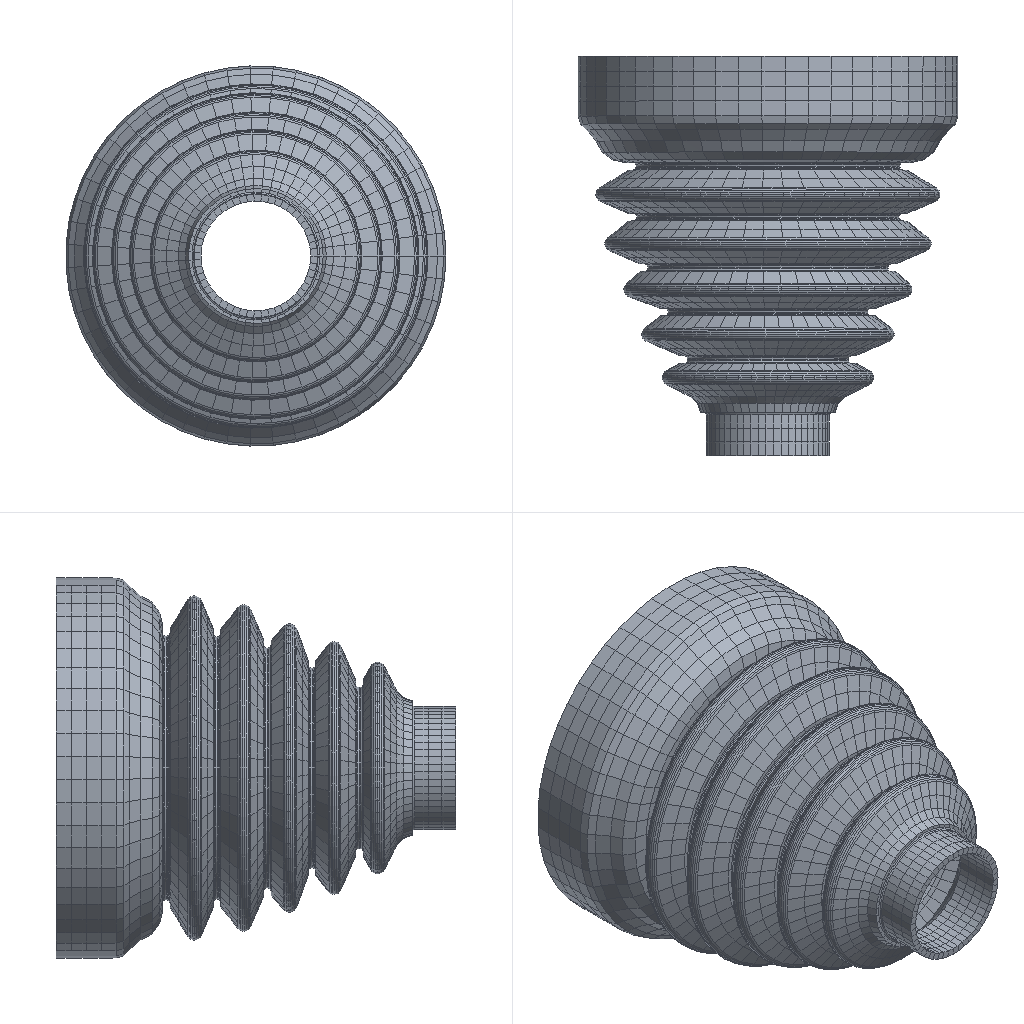Simulation study | abaqus
Set-up summary:
category,name,step,type,value,unit,region
solver,abaqus,,Abaqus/CAE 2024
units,unstated,,unstated
analysis,Step-1,,static,nlgeom=True; time_period=1
analysis,Step-2,,static,nlgeom=True; time_period=1
mesh,nodes,,,62019
mesh,elements,,,11731
element_type,C3D20H,,,11730
element_type,CONN3D2,,,1
material,MATERIAL-1,,behaviors,hyperelastic; viscoelastic
section,MATERIAL-1,,solid section,,,SET-2
bc,BC-5,Step-1,fixed,"[dofs=rx,ry,rz,x,y,z n=6]",,_PickedSet80
bc,BC-5-Copy,Step-1,fixed,"[dofs=rx,ry,rz,x,y,z n=6]",,_PickedSet79
bc,BC-5,Step-2,displacement,0.75 [dofs=ry],,_PickedSet80
bc,BC-5-Copy,Step-2,displacement,0.75 [dofs=ry],,_PickedSet79
bc,BC-7,Step-2,fixed,"[dofs=rx,rz,x,y,z n=5]",,_PickedSet78
bc,BC-7,Step-2,displacement,0.75 [dofs=ry],,_PickedSet78
contact,Int-2,initial,general contact,interaction=INTPROP-1; friction=0.3; behavior=hard
constraint,connector section,,,1
constraint,coupling,,,2
Abaqus input file, long lists of numbers shortened:
*Heading
** Job name: deck Model name: Job-1-Copy-Copy
** Generated by: Abaqus/CAE 2024
*Preprint, echo=NO, model=NO, history=NO, contact=NO
**
** PARTS
**
*Part, name=PART-1-1
*Node
      1,         14.5,        -122.,           0.
      2,         14.5,  -109.9,           0.
** (62014 more lines like these left out)
*Element, type=C3D20H
    1,    156,      1,    157,    196,    485,    330,    486,    525,  62020,  62019,  62018,  62017,  62021,  62022,  62023,
        62024,  62026,  62025,  62027,  62028
** (23458 more lines like these left out)
*Nset, nset=SET-1, generate
     1,  16779,      1
*Elset, elset=SET-1, generate
     1,  11730,      1
*Nset, nset=SET-2, generate
     1,  16779,      1
*Elset, elset=SET-2, generate
     1,  11730,      1
** Section: Section-1-SET-2
*Solid Section, elset=SET-2, material=MATERIAL-1
,
*End Part
**
**
** ASSEMBLY
**
*Assembly, name=Assembly
**
*Instance, name=PART-1-1, part=PART-1-1
*End Instance
**
*Node
      3,           0.,           0.,           0.
*Node
      1,           0.,        -116.,           0.
      2,           0.,         -25.,           0.
*Element, type=CONN3D2
1, 1, 3
*Connector Section, elset=Wire-1-Set-2
Hinge,
"Datum csys-1",
*Nset, nset=M_SET-1
 1,
*Nset, nset=M_SET-8
 1,
*Nset, nset=M_SET-10
 2,
*Nset, nset=M_SET-14
 1,
*Nset, nset=M_SET-16
 2,
*Nset, nset=M_SET-21, instance=PART-1-1
    53,    54,   170,   171,   172,   382,   383,   499,   500,   501,   711,   712,   828,   829,   830,  1040
  1041,  1157,  1158,  1159,  1369,  1370,  1486,  1487,  1488,  1698,  1699,  1815,  1816,  1817,  2027,  2028
** (14 more lines like these left out)
*Elset, elset=M_SET-21, instance=PART-1-1
    91,    92,   120,   121,   321,   322,   350,   351,   551,   552,   580,   581,   781,   782,   810,   811
  1011,  1012,  1040,  1041,  1241,  1242,  1270,  1271,  1471,  1472,  1500,  1501,  1701,  1702,  1730,  1731
** (11 more lines like these left out)
*Nset, nset=M_SET-27
 1,
*Nset, nset=M_SET-29
 2,
*Nset, nset=SET-3, instance=PART-1-1
    55,    56,   173,   174,   175,   384,   385,   502,   503,   504,   713,   714,   831,   832,   833,  1042
  1043,  1160,  1161,  1162,  1371,  1372,  1489,  1490,  1491,  1700,  1701,  1818,  1819,  1820,  2029,  2030
** (14 more lines like these left out)
*Elset, elset=SET-3, instance=PART-1-1
    91,    92,   120,   121,   321,   322,   350,   351,   551,   552,   580,   581,   781,   782,   810,   811
  1011,  1012,  1040,  1041,  1241,  1242,  1270,  1271,  1471,  1472,  1500,  1501,  1701,  1702,  1730,  1731
** (11 more lines like these left out)
*Nset, nset=SET-4
 1,
*Nset, nset=SET-5, instance=PART-1-1, generate
     1,  16779,      1
*Nset, nset=SET-5
 1,
*Elset, elset=SET-5, instance=PART-1-1, generate
     1,  11730,      1
*Nset, nset=SET-7, instance=PART-1-1
     1,     2,   157,   158,   159,   330,   331,   486,   487,   488,   659,   660,   815,   816,   817,   988
   989,  1144,  1145,  1146,  1317,  1318,  1473,  1474,  1475,  1646,  1647,  1802,  1803,  1804,  1975,  1976
** (14 more lines like these left out)
*Elset, elset=SET-7, instance=PART-1-1
     1,     2,   110,   177,   231,   232,   340,   407,   461,   462,   570,   637,   691,   692,   800,   867
   921,   922,  1030,  1097,  1151,  1152,  1260,  1327,  1381,  1382,  1490,  1557,  1611,  1612,  1720,  1787
** (11 more lines like these left out)
*Nset, nset=SET-12
 1,
*Nset, nset=SET-13, instance=PART-1-1
    53,    54,   170,   171,   172,   382,   383,   499,   500,   501,   711,   712,   828,   829,   830,  1040
  1041,  1157,  1158,  1159,  1369,  1370,  1486,  1487,  1488,  1698,  1699,  1815,  1816,  1817,  2027,  2028
** (14 more lines like these left out)
*Elset, elset=SET-13, instance=PART-1-1
    91,    92,   120,   121,   321,   322,   350,   351,   551,   552,   580,   581,   781,   782,   810,   811
  1011,  1012,  1040,  1041,  1241,  1242,  1270,  1271,  1471,  1472,  1500,  1501,  1701,  1702,  1730,  1731
** (11 more lines like these left out)
*Nset, nset=SET-18
 1,
*Nset, nset=SET-19, instance=PART-1-1
     1,     2,   157,   158,   159,   330,   331,   486,   487,   488,   659,   660,   815,   816,   817,   988
   989,  1144,  1145,  1146,  1317,  1318,  1473,  1474,  1475,  1646,  1647,  1802,  1803,  1804,  1975,  1976
** (14 more lines like these left out)
*Elset, elset=SET-19, instance=PART-1-1
     1,     2,   110,   177,   231,   232,   340,   407,   461,   462,   570,   637,   691,   692,   800,   867
   921,   922,  1030,  1097,  1151,  1152,  1260,  1327,  1381,  1382,  1490,  1557,  1611,  1612,  1720,  1787
** (11 more lines like these left out)
*Nset, nset=SET-20, instance=PART-1-1
    53,    54,   170,   171,   172,   382,   383,   499,   500,   501,   711,   712,   828,   829,   830,  1040
  1041,  1157,  1158,  1159,  1369,  1370,  1486,  1487,  1488,  1698,  1699,  1815,  1816,  1817,  2027,  2028
** (14 more lines like these left out)
*Elset, elset=SET-20, instance=PART-1-1
    91,    92,   120,   121,   321,   322,   350,   351,   551,   552,   580,   581,   781,   782,   810,   811
  1011,  1012,  1040,  1041,  1241,  1242,  1270,  1271,  1471,  1472,  1500,  1501,  1701,  1702,  1730,  1731
** (11 more lines like these left out)
*Nset, nset=SET-23, instance=PART-1-1
    53,    54,   170,   171,   172,   382,   383,   499,   500,   501,   711,   712,   828,   829,   830,  1040
  1041,  1157,  1158,  1159,  1369,  1370,  1486,  1487,  1488,  1698,  1699,  1815,  1816,  1817,  2027,  2028
** (14 more lines like these left out)
*Elset, elset=SET-23, instance=PART-1-1
    91,    92,   120,   121,   321,   322,   350,   351,   551,   552,   580,   581,   781,   782,   810,   811
  1011,  1012,  1040,  1041,  1241,  1242,  1270,  1271,  1471,  1472,  1500,  1501,  1701,  1702,  1730,  1731
** (11 more lines like these left out)
*Nset, nset=SET-24, instance=PART-1-1
     1,     2,   157,   158,   159,   330,   331,   486,   487,   488,   659,   660,   815,   816,   817,   988
   989,  1144,  1145,  1146,  1317,  1318,  1473,  1474,  1475,  1646,  1647,  1802,  1803,  1804,  1975,  1976
** (14 more lines like these left out)
*Elset, elset=SET-24, instance=PART-1-1
     1,     2,   110,   177,   231,   232,   340,   407,   461,   462,   570,   637,   691,   692,   800,   867
   921,   922,  1030,  1097,  1151,  1152,  1260,  1327,  1381,  1382,  1490,  1557,  1611,  1612,  1720,  1787
** (11 more lines like these left out)
*Nset, nset=SET-31, instance=PART-1-1, generate
     1,  16779,      1
*Nset, nset=SET-31
 1, 2
*Elset, elset=SET-31, instance=PART-1-1, generate
     1,  11730,      1
*Nset, nset=SET-44
 1,
*Nset, nset=S_SET-1, instance=PART-1-1
     1,     2,   157,   158,   159,   330,   331,   486,   487,   488,   659,   660,   815,   816,   817,   988
   989,  1144,  1145,  1146,  1317,  1318,  1473,  1474,  1475,  1646,  1647,  1802,  1803,  1804,  1975,  1976
** (14 more lines like these left out)
*Elset, elset=S_SET-1, instance=PART-1-1
     1,     2,   110,   177,   231,   232,   340,   407,   461,   462,   570,   637,   691,   692,   800,   867
   921,   922,  1030,  1097,  1151,  1152,  1260,  1327,  1381,  1382,  1490,  1557,  1611,  1612,  1720,  1787
** (11 more lines like these left out)
*Nset, nset=S_SET-8, instance=PART-1-1
     1,     2,   157,   158,   159,   330,   331,   486,   487,   488,   659,   660,   815,   816,   817,   988
   989,  1144,  1145,  1146,  1317,  1318,  1473,  1474,  1475,  1646,  1647,  1802,  1803,  1804,  1975,  1976
** (14 more lines like these left out)
*Elset, elset=S_SET-8, instance=PART-1-1
     1,     2,   110,   177,   231,   232,   340,   407,   461,   462,   570,   637,   691,   692,   800,   867
   921,   922,  1030,  1097,  1151,  1152,  1260,  1327,  1381,  1382,  1490,  1557,  1611,  1612,  1720,  1787
** (11 more lines like these left out)
*Nset, nset=S_SET-10, instance=PART-1-1
    53,    54,   170,   171,   172,   382,   383,   499,   500,   501,   711,   712,   828,   829,   830,  1040
  1041,  1157,  1158,  1159,  1369,  1370,  1486,  1487,  1488,  1698,  1699,  1815,  1816,  1817,  2027,  2028
** (14 more lines like these left out)
*Elset, elset=S_SET-10, instance=PART-1-1
    91,    92,   120,   121,   321,   322,   350,   351,   551,   552,   580,   581,   781,   782,   810,   811
  1011,  1012,  1040,  1041,  1241,  1242,  1270,  1271,  1471,  1472,  1500,  1501,  1701,  1702,  1730,  1731
** (11 more lines like these left out)
*Nset, nset=S_SET-14, instance=PART-1-1
     1,     2,   157,   158,   159,   330,   331,   486,   487,   488,   659,   660,   815,   816,   817,   988
   989,  1144,  1145,  1146,  1317,  1318,  1473,  1474,  1475,  1646,  1647,  1802,  1803,  1804,  1975,  1976
** (14 more lines like these left out)
*Elset, elset=S_SET-14, instance=PART-1-1
     1,     2,   110,   177,   231,   232,   340,   407,   461,   462,   570,   637,   691,   692,   800,   867
   921,   922,  1030,  1097,  1151,  1152,  1260,  1327,  1381,  1382,  1490,  1557,  1611,  1612,  1720,  1787
** (11 more lines like these left out)
*Nset, nset=S_SET-16, instance=PART-1-1
    53,    54,   170,   171,   172,   382,   383,   499,   500,   501,   711,   712,   828,   829,   830,  1040
  1041,  1157,  1158,  1159,  1369,  1370,  1486,  1487,  1488,  1698,  1699,  1815,  1816,  1817,  2027,  2028
** (14 more lines like these left out)
*Elset, elset=S_SET-16, instance=PART-1-1
    91,    92,   120,   121,   321,   322,   350,   351,   551,   552,   580,   581,   781,   782,   810,   811
  1011,  1012,  1040,  1041,  1241,  1242,  1270,  1271,  1471,  1472,  1500,  1501,  1701,  1702,  1730,  1731
** (11 more lines like these left out)
*Nset, nset=S_SET-21
 2,
*Nset, nset=S_SET-27, instance=PART-1-1
     1,     2,   157,   158,   159,   330,   331,   486,   487,   488,   659,   660,   815,   816,   817,   988
   989,  1144,  1145,  1146,  1317,  1318,  1473,  1474,  1475,  1646,  1647,  1802,  1803,  1804,  1975,  1976
** (14 more lines like these left out)
*Elset, elset=S_SET-27, instance=PART-1-1
     1,     2,   110,   177,   231,   232,   340,   407,   461,   462,   570,   637,   691,   692,   800,   867
   921,   922,  1030,  1097,  1151,  1152,  1260,  1327,  1381,  1382,  1490,  1557,  1611,  1612,  1720,  1787
** (11 more lines like these left out)
*Nset, nset=S_SET-29, instance=PART-1-1
    53,    54,   170,   171,   172,   382,   383,   499,   500,   501,   711,   712,   828,   829,   830,  1040
  1041,  1157,  1158,  1159,  1369,  1370,  1486,  1487,  1488,  1698,  1699,  1815,  1816,  1817,  2027,  2028
** (14 more lines like these left out)
*Elset, elset=S_SET-29, instance=PART-1-1
    91,    92,   120,   121,   321,   322,   350,   351,   551,   552,   580,   581,   781,   782,   810,   811
  1011,  1012,  1040,  1041,  1241,  1242,  1270,  1271,  1471,  1472,  1500,  1501,  1701,  1702,  1730,  1731
** (11 more lines like these left out)
*Nset, nset=Wire-1-Set-2
 1, 3
*Elset, elset=Wire-1-Set-2
 1,
*Nset, nset=S_SET-27_CNS_, internal, instance=PART-1-1
     1,     2,   157,   158,   159,   330,   331,   486,   487,   488,   659,   660,   815,   816,   817,   988
   989,  1144,  1145,  1146,  1317,  1318,  1473,  1474,  1475,  1646,  1647,  1802,  1803,  1804,  1975,  1976
** (14 more lines like these left out)
*Nset, nset=S_SET-29_CNS_, internal, instance=PART-1-1
    53,    54,   170,   171,   172,   382,   383,   499,   500,   501,   711,   712,   828,   829,   830,  1040
  1041,  1157,  1158,  1159,  1369,  1370,  1486,  1487,  1488,  1698,  1699,  1815,  1816,  1817,  2027,  2028
** (14 more lines like these left out)
*Nset, nset=_PickedSet68, internal
 2,
*Nset, nset=_PickedSet73, internal
 3,
*Nset, nset=_PickedSet77, internal
 1,
*Nset, nset=_PickedSet78, internal
 1,
*Nset, nset=_PickedSet79, internal
 2,
*Nset, nset=_PickedSet80, internal
 3,
*Elset, elset=_PickedSet81, internal
 1,
*Elset, elset=_SURF-1_S3, internal, instance=PART-1-1
     1,     5,     8,    14,    19,    20,    26,    33,    53,    56,    57,    59,    64,    89,    93,    95
    98,   100,   101,   106,   113,   115,   118,   133,   144,   152,   160,   161,   162,   163,   165,   167
** (139 more lines like these left out)
*Elset, elset=_SURF-1_S4, internal, instance=PART-1-1
     1,     2,     6,     7,    10,    17,    18,    21,    27,    31,    43,    45,    47,    52,    55,    58
    62,    66,    69,    77,    81,    87,    88,    90,    91,    92,    96,   104,   107,   109,   110,   114
** (180 more lines like these left out)
*Elset, elset=_SURF-1_S5, internal, instance=PART-1-1
     4,     9,    11,    15,    16,    24,    29,    32,    34,    36,    37,    42,    46,    49,    53,    60
    61,    67,    73,    82,    85,    89,    93,    95,   102,   103,   111,   113,   121,   130,   132,   137
** (142 more lines like these left out)
*Elset, elset=_SURF-1_S6, internal, instance=PART-1-1
     1,     2,     3,     5,     6,     7,    13,    22,    30,    39,    44,    50,    51,    52,    54,    63
    65,    68,    70,    71,    74,    78,    79,    83,    84,    86,    88,    90,    91,    92,    99,   109
** (158 more lines like these left out)
*Elset, elset=_SURF-2_S3, internal, instance=PART-1-1
     1,     5,     8,    14,    19,    20,    26,    33,    53,    56,    57,    59,    64,    89,    93,    95
    98,   100,   101,   106,   113,   115,   118,   133,   144,   152,   160,   161,   162,   163,   165,   167
** (139 more lines like these left out)
*Elset, elset=_SURF-2_S4, internal, instance=PART-1-1
     1,     2,     6,     7,    10,    17,    18,    21,    27,    31,    43,    45,    47,    52,    55,    58
    62,    66,    69,    77,    81,    87,    88,    90,    91,    92,    96,   104,   107,   109,   110,   114
** (180 more lines like these left out)
*Elset, elset=_SURF-2_S5, internal, instance=PART-1-1
     4,     9,    11,    15,    16,    24,    29,    32,    34,    36,    37,    42,    46,    49,    53,    60
    61,    67,    73,    82,    85,    89,    93,    95,   102,   103,   111,   113,   121,   130,   132,   137
** (142 more lines like these left out)
*Elset, elset=_SURF-2_S6, internal, instance=PART-1-1
     1,     2,     3,     5,     6,     7,    13,    22,    30,    39,    44,    50,    51,    52,    54,    63
    65,    68,    70,    71,    74,    78,    79,    83,    84,    86,    88,    90,    91,    92,    99,   109
** (158 more lines like these left out)
*Elset, elset=_SURF-1_S3_1, internal, instance=PART-1-1
     1,     5,     8,    14,    19,    20,    26,    33,    53,    56,    57,    59,    64,    89,    93,    95
    98,   100,   101,   106,   113,   115,   118,   133,   144,   152,   160,   161,   162,   163,   165,   167
** (139 more lines like these left out)
*Elset, elset=_SURF-1_S4_1, internal, instance=PART-1-1
     1,     2,     6,     7,    10,    17,    18,    21,    27,    31,    43,    45,    47,    52,    55,    58
    62,    66,    69,    77,    81,    87,    88,    90,    91,    92,    96,   104,   107,   109,   110,   114
** (180 more lines like these left out)
*Elset, elset=_SURF-1_S6_1, internal, instance=PART-1-1
     1,     2,     3,     5,     6,     7,    13,    22,    30,    39,    44,    50,    51,    52,    54,    63
    65,    68,    70,    71,    74,    78,    79,    83,    84,    86,    88,    90,    91,    92,    99,   109
** (158 more lines like these left out)
*Elset, elset=_SURF-1_S5_1, internal, instance=PART-1-1
     4,     9,    11,    15,    16,    24,    29,    32,    34,    36,    37,    42,    46,    49,    53,    60
    61,    67,    73,    82,    85,    89,    93,    95,   102,   103,   111,   113,   121,   130,   132,   137
** (142 more lines like these left out)
*Surface, type=ELEMENT, name=SURF-1
_SURF-1_S3_1, S3
_SURF-1_S4_1, S4
_SURF-1_S6_1, S6
_SURF-1_S5_1, S5
*Elset, elset=_SURF-2_S3_1, internal, instance=PART-1-1
     1,     5,     8,    14,    19,    20,    26,    33,    53,    56,    57,    59,    64,    89,    93,    95
    98,   100,   101,   106,   113,   115,   118,   133,   144,   152,   160,   161,   162,   163,   165,   167
** (139 more lines like these left out)
*Elset, elset=_SURF-2_S4_1, internal, instance=PART-1-1
     1,     2,     6,     7,    10,    17,    18,    21,    27,    31,    43,    45,    47,    52,    55,    58
    62,    66,    69,    77,    81,    87,    88,    90,    91,    92,    96,   104,   107,   109,   110,   114
** (180 more lines like these left out)
*Elset, elset=_SURF-2_S6_1, internal, instance=PART-1-1
     1,     2,     3,     5,     6,     7,    13,    22,    30,    39,    44,    50,    51,    52,    54,    63
    65,    68,    70,    71,    74,    78,    79,    83,    84,    86,    88,    90,    91,    92,    99,   109
** (158 more lines like these left out)
*Elset, elset=_SURF-2_S5_1, internal, instance=PART-1-1
     4,     9,    11,    15,    16,    24,    29,    32,    34,    36,    37,    42,    46,    49,    53,    60
    61,    67,    73,    82,    85,    89,    93,    95,   102,   103,   111,   113,   121,   130,   132,   137
** (142 more lines like these left out)
*Surface, type=ELEMENT, name=SURF-2
_SURF-2_S3_1, S3
_SURF-2_S4_1, S4
_SURF-2_S6_1, S6
_SURF-2_S5_1, S5
*Surface, type=NODE, name=S_SET-27_CNS__CNS_, internal
S_SET-27_CNS_, 1.
*Surface, type=NODE, name=S_SET-29_CNS__CNS_, internal
S_SET-29_CNS_, 1.
*Orientation, name="Datum csys-1"
          1.,           0.,           0.,           0.,           1.,           0.
1, 0.
** Constraint: CONSTRAINT-1
*Coupling, constraint name=CONSTRAINT-1, ref node=M_SET-27, surface=S_SET-27_CNS__CNS_
*Kinematic
** Constraint: CONSTRAINT-2
*Coupling, constraint name=CONSTRAINT-2, ref node=M_SET-29, surface=S_SET-29_CNS__CNS_
*Kinematic
1, 1
2, 2
3, 3
4, 4
6, 6
*End Assembly
*Amplitude, name=AMP-1, definition=SMOOTH STEP
             0.,              0.,           0.175,           0.175
*Amplitude, name=AMP-2, definition=SMOOTH STEP
             0.,              0.,              1.,              1.
*Amplitude, name=AMP-3, definition=SMOOTH STEP
             0.,              0.,             0.1,            0.08
*Amplitude, name=Amp-4
             0.,              0.,              1.,              1.
**
** MATERIALS
**
*Material, name=MATERIAL-1
*Hyperelastic, mooney-rivlin, moduli=LONG TERM
 0.8073, 0.1689,  0.001
*Viscoelastic, frequency=PRONY
 0.05,   0., 0.01
**
** INTERACTION PROPERTIES
**
*Surface Interaction, name=INTPROP-1
1.,
*Friction, slip tolerance=0.005
 0.3,
*Surface Behavior, pressure-overclosure=HARD
**
** INTERACTIONS
**
** Interaction: Int-2
*Contact
*Contact Inclusions, ALL EXTERIOR
*Contact Property Assignment
 ,  , INTPROP-1
** ----------------------------------------------------------------
**
** STEP: Step-1
**
*Step, name=Step-1, nlgeom=YES, inc=10000
*Static, stabilize=0.0002, allsdtol=0.05, continue=NO
0.1, 1., 1e-06, 0.1
**
** BOUNDARY CONDITIONS
**
** Name: BC-2 Type: Connector displacement
*Connector Motion, amplitude=Amp-4
Wire-1-Set-2, 4, 0.2181
** Name: BC-5 Type: Displacement/Rotation
*Boundary
_PickedSet80, 1, 1
_PickedSet80, 2, 2
_PickedSet80, 3, 3
_PickedSet80, 4, 4
_PickedSet80, 5, 5
_PickedSet80, 6, 6
** Name: BC-5-Copy Type: Displacement/Rotation
*Boundary
_PickedSet79, 1, 1
_PickedSet79, 2, 2
_PickedSet79, 3, 3
_PickedSet79, 4, 4
_PickedSet79, 5, 5
_PickedSet79, 6, 6
**
** OUTPUT REQUESTS
**
*Restart, write, number interval=1, time marks=NO
**
** FIELD OUTPUT: F-Output-1
**
*Output, field, variable=PRESELECT
**
** HISTORY OUTPUT: H-Output-2
**
*Output, history
*Energy Output
ALLAE, ALLCD, ALLDMD, ALLFD, ALLIE, ALLKE, ALLPD, ALLSE, ALLVD, ALLWK, ETOTAL
*End Step
** ----------------------------------------------------------------
**
** STEP: Step-2
**
*Step, name=Step-2, nlgeom=YES, inc=10000
*Static
0.01, 1., 1e-06, 0.1
**
** BOUNDARY CONDITIONS
**
** Name: BC-5 Type: Displacement/Rotation
*Boundary
_PickedSet80, 5, 5, 0.75
** Name: BC-5-Copy Type: Displacement/Rotation
*Boundary
_PickedSet79, 5, 5, 0.75
** Name: BC-7 Type: Displacement/Rotation
*Boundary
_PickedSet78, 1, 1
_PickedSet78, 2, 2
_PickedSet78, 3, 3
_PickedSet78, 4, 4
_PickedSet78, 5, 5, 0.75
_PickedSet78, 6, 6
**
** INTERACTIONS
**
** Interaction: Int-3
*Model Change, remove
_PickedSet81,
**
** OUTPUT REQUESTS
**
*Restart, write, frequency=0
**
** FIELD OUTPUT: F-Output-1
**
*Output, field, variable=PRESELECT
**
** HISTORY OUTPUT: H-Output-2
**
*Output, history
*Energy Output
ALLAE, ALLCD, ALLDMD, ALLFD, ALLIE, ALLKE, ALLPD, ALLSE, ALLVD, ALLWK, ETOTAL
*End Step
Results summary:
result,odb.job_status,,,JOB_STATUS_COMPLETED_SUCCESSFULLY,"consistent, unstated (Abaqus has no unit system)"
result,steps[0].procedure,Step-1,,*STATIC,"consistent, unstated (Abaqus has no unit system)"
result,steps[0].time_period,Step-1,,1,"consistent, unstated (Abaqus has no unit system)"
result,steps[0].n_frames,Step-1,,13,"consistent, unstated (Abaqus has no unit system)"
result,steps[0].last_frame.id,Step-1,,12,"consistent, unstated (Abaqus has no unit system)"
result,steps[0].last_frame.value,Step-1,,1,"consistent, unstated (Abaqus has no unit system)"
result,steps[0].last_frame.description,Step-1,,Increment     12: Step Time =    1.000,"consistent, unstated (Abaqus has no unit system)"
result,steps[0].completed,Step-1,,True,"consistent, unstated (Abaqus has no unit system)"
result,steps[0].max_U_magnitude,Step-1,,26.788,"consistent, unstated (Abaqus has no unit system)"
result,steps[0].max_S_mises,Step-1,,0.9619,"consistent, unstated (Abaqus has no unit system)"
result,steps[0].RF_sum[1],Step-1,,-3.23748e-06,"consistent, unstated (Abaqus has no unit system)"
result,steps[0].RF_sum[2],Step-1,,0.00677,"consistent, unstated (Abaqus has no unit system)"
result,steps[0].RF_sum[3],Step-1,,0.02577,"consistent, unstated (Abaqus has no unit system)"
result,steps[1].procedure,Step-2,,*STATIC,"consistent, unstated (Abaqus has no unit system)"
result,steps[1].time_period,Step-2,,1,"consistent, unstated (Abaqus has no unit system)"
result,steps[1].n_frames,Step-2,,19,"consistent, unstated (Abaqus has no unit system)"
result,steps[1].last_frame.id,Step-2,,18,"consistent, unstated (Abaqus has no unit system)"
result,steps[1].last_frame.value,Step-2,,1,"consistent, unstated (Abaqus has no unit system)"
result,steps[1].last_frame.description,Step-2,,Increment     18: Step Time =    1.000,"consistent, unstated (Abaqus has no unit system)"
result,steps[1].completed,Step-2,,True,"consistent, unstated (Abaqus has no unit system)"
result,steps[1].max_U_magnitude,Step-2,,36.848,"consistent, unstated (Abaqus has no unit system)"
result,steps[1].max_S_mises,Step-2,,0.2311,"consistent, unstated (Abaqus has no unit system)"
result,steps[1].RF_sum[1],Step-2,,-1.84774e-06,"consistent, unstated (Abaqus has no unit system)"
result,steps[1].RF_sum[2],Step-2,,0.0005963,"consistent, unstated (Abaqus has no unit system)"
result,steps[1].RF_sum[3],Step-2,,1.49012e-06,"consistent, unstated (Abaqus has no unit system)"